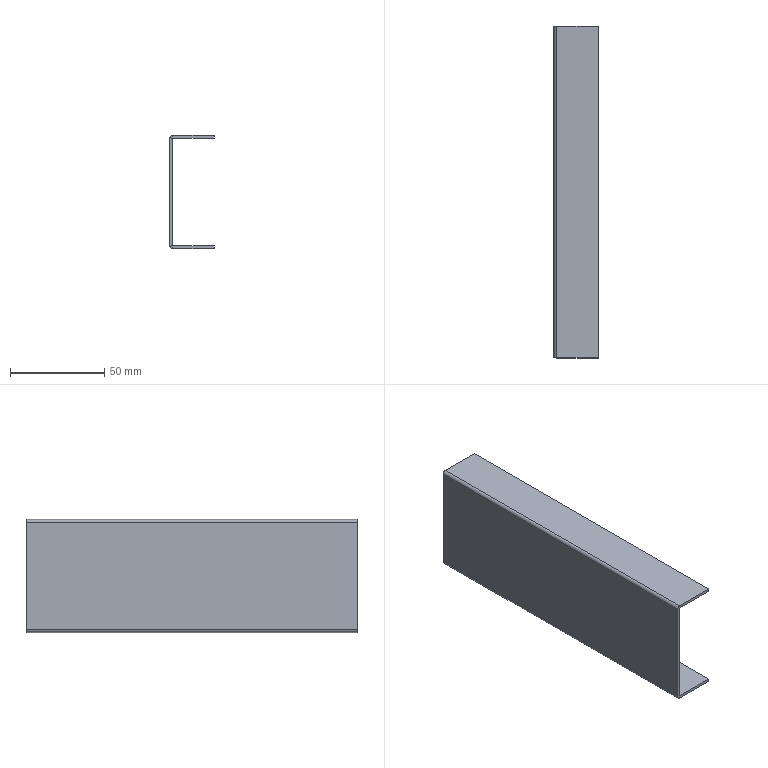Part | SolidWorks | features SplitBody 1 | 1 solid | 22 faces | box 23.5 x 176 x 60 mm | volume 27263 mm3 | plane 18 | cylinder 4 | commonest cylinder face diameters 0.2 x2 3.2 x2
STEP:
#1=CARTESIAN_POINT('',(3.,1360.,273.4));
#2=VERTEX_POINT('',#1);
#3=CARTESIAN_POINT('',(1.5,1360.,273.4));
#4=VERTEX_POINT('',#3);
#5=CARTESIAN_POINT('',(3.,1360.,273.4));
#6=DIRECTION('',(-1.,0.,0.));
#7=VECTOR('',#6,1000.);
#8=LINE('',#5,#7);
#9=EDGE_CURVE('',#2,#4,#8,.T.);
#10=ORIENTED_EDGE('',*,*,#9,.T.);
#11=CARTESIAN_POINT('',(1.5,1360.,216.6));
#12=VERTEX_POINT('',#11);
#13=CARTESIAN_POINT('',(1.5,1360.,0.));
#14=DIRECTION('',(0.,0.,1.));
#15=VECTOR('',#14,1000.);
#16=LINE('',#13,#15);
#17=EDGE_CURVE('',#12,#4,#16,.T.);
#18=ORIENTED_EDGE('',*,*,#17,.F.);
#19=CARTESIAN_POINT('',(3.,1360.,216.6));
#20=VERTEX_POINT('',#19);
#21=CARTESIAN_POINT('',(3.,1360.,216.6));
#22=DIRECTION('',(-1.,0.,0.));
#23=VECTOR('',#22,1000.);
#24=LINE('',#21,#23);
#25=EDGE_CURVE('',#20,#12,#24,.T.);
#26=ORIENTED_EDGE('',*,*,#25,.F.);
#27=CARTESIAN_POINT('',(3.,1360.,275.));
#28=DIRECTION('',(0.,0.,1.));
#29=VECTOR('',#28,1000.);
#30=LINE('',#27,#29);
#31=EDGE_CURVE('',#20,#2,#30,.T.);
#32=ORIENTED_EDGE('',*,*,#31,.T.);
#33=EDGE_LOOP('',(#10,#18,#26,#32));
#34=FACE_OUTER_BOUND('',#33,.T.);
#35=CARTESIAN_POINT('',(1.5,1360.,275.));
#36=DIRECTION('',(0.,1.,0.));
#37=DIRECTION('',(-1.,0.,0.));
#38=AXIS2_PLACEMENT_3D('',#35,#36,#37);
#39=PLANE('',#38);
#40=ADVANCED_FACE('',(#34),#39,.F.);
#41=CARTESIAN_POINT('',(3.,1536.,273.4));
#42=VERTEX_POINT('',#41);
#43=CARTESIAN_POINT('',(1.5,1536.,273.4));
#44=VERTEX_POINT('',#43);
#45=CARTESIAN_POINT('',(3.,1536.,273.4));
#46=DIRECTION('',(-1.,0.,0.));
#47=VECTOR('',#46,1000.);
#48=LINE('',#45,#47);
#49=EDGE_CURVE('',#42,#44,#48,.T.);
#50=ORIENTED_EDGE('',*,*,#49,.F.);
#51=CARTESIAN_POINT('',(3.,1536.,216.6));
#52=VERTEX_POINT('',#51);
#53=CARTESIAN_POINT('',(3.,1536.,216.5));
#54=DIRECTION('',(0.,0.,-1.));
#55=VECTOR('',#54,1000.);
#56=LINE('',#53,#55);
#57=EDGE_CURVE('',#42,#52,#56,.T.);
#58=ORIENTED_EDGE('',*,*,#57,.T.);
#59=CARTESIAN_POINT('',(1.5,1536.,216.6));
#60=VERTEX_POINT('',#59);
#61=CARTESIAN_POINT('',(1.5,1536.,216.6));
#62=DIRECTION('',(-1.,0.,0.));
#63=VECTOR('',#62,1000.);
#64=LINE('',#61,#63);
#65=EDGE_CURVE('',#52,#60,#64,.T.);
#66=ORIENTED_EDGE('',*,*,#65,.T.);
#67=CARTESIAN_POINT('',(1.5,1536.,0.));
#68=DIRECTION('',(0.,0.,-1.));
#69=VECTOR('',#68,1000.);
#70=LINE('',#67,#69);
#71=EDGE_CURVE('',#44,#60,#70,.T.);
#72=ORIENTED_EDGE('',*,*,#71,.F.);
#73=EDGE_LOOP('',(#50,#58,#66,#72));
#74=FACE_OUTER_BOUND('',#73,.T.);
#75=CARTESIAN_POINT('',(1.5,1536.,216.5));
#76=DIRECTION('',(0.,-1.,0.));
#77=DIRECTION('',(1.,0.,0.));
#78=AXIS2_PLACEMENT_3D('',#75,#76,#77);
#79=PLANE('',#78);
#80=ADVANCED_FACE('',(#74),#79,.F.);
#81=CARTESIAN_POINT('',(1.5,1360.,273.4));
#82=DIRECTION('',(0.,1.,0.));
#83=VECTOR('',#82,1000.);
#84=LINE('',#81,#83);
#85=EDGE_CURVE('',#4,#44,#84,.T.);
#86=ORIENTED_EDGE('',*,*,#85,.T.);
#87=ORIENTED_EDGE('',*,*,#71,.T.);
#88=CARTESIAN_POINT('',(1.5,1536.,216.6));
#89=DIRECTION('',(0.,1.,0.));
#90=VECTOR('',#89,1000.);
#91=LINE('',#88,#90);
#92=EDGE_CURVE('',#12,#60,#91,.T.);
#93=ORIENTED_EDGE('',*,*,#92,.F.);
#94=ORIENTED_EDGE('',*,*,#17,.T.);
#95=EDGE_LOOP('',(#86,#87,#93,#94));
#96=FACE_OUTER_BOUND('',#95,.T.);
#97=CARTESIAN_POINT('',(1.5,0.,0.));
#98=DIRECTION('',(1.,0.,0.));
#99=DIRECTION('',(0.,0.,-1.));
#100=AXIS2_PLACEMENT_3D('',#97,#98,#99);
#101=PLANE('',#100);
#102=ADVANCED_FACE('',(#96),#101,.F.);
#103=ORIENTED_EDGE('',*,*,#57,.F.);
#104=CARTESIAN_POINT('',(3.,1360.,273.4));
#105=DIRECTION('',(0.,1.,0.));
#106=VECTOR('',#105,1000.);
#107=LINE('',#104,#106);
#108=EDGE_CURVE('',#2,#42,#107,.T.);
#109=ORIENTED_EDGE('',*,*,#108,.F.);
#110=ORIENTED_EDGE('',*,*,#31,.F.);
#111=CARTESIAN_POINT('',(3.,1536.,216.6));
#112=DIRECTION('',(0.,-1.,0.));
#113=VECTOR('',#112,1000.);
#114=LINE('',#111,#113);
#115=EDGE_CURVE('',#52,#20,#114,.T.);
#116=ORIENTED_EDGE('',*,*,#115,.F.);
#117=EDGE_LOOP('',(#103,#109,#110,#116));
#118=FACE_OUTER_BOUND('',#117,.T.);
#119=CARTESIAN_POINT('',(3.,0.,0.));
#120=DIRECTION('',(1.,0.,0.));
#121=DIRECTION('',(0.,0.,-1.));
#122=AXIS2_PLACEMENT_3D('',#119,#120,#121);
#123=PLANE('',#122);
#124=ADVANCED_FACE('',(#118),#123,.T.);
#125=CARTESIAN_POINT('',(3.1,1536.,216.5));
#126=VERTEX_POINT('',#125);
#127=CARTESIAN_POINT('',(3.1,1536.,215.));
#128=VERTEX_POINT('',#127);
#129=CARTESIAN_POINT('',(3.1,1536.,216.5));
#130=DIRECTION('',(0.,0.,-1.));
#131=VECTOR('',#130,1000.);
#132=LINE('',#129,#131);
#133=EDGE_CURVE('',#126,#128,#132,.T.);
#134=ORIENTED_EDGE('',*,*,#133,.F.);
#135=CARTESIAN_POINT('',(25.,1536.,216.5));
#136=VERTEX_POINT('',#135);
#137=CARTESIAN_POINT('',(25.,1536.,216.5));
#138=DIRECTION('',(-1.,0.,0.));
#139=VECTOR('',#138,1000.);
#140=LINE('',#137,#139);
#141=EDGE_CURVE('',#136,#126,#140,.T.);
#142=ORIENTED_EDGE('',*,*,#141,.F.);
#143=CARTESIAN_POINT('',(25.,1536.,215.));
#144=VERTEX_POINT('',#143);
#145=CARTESIAN_POINT('',(25.,1536.,216.5));
#146=DIRECTION('',(0.,0.,-1.));
#147=VECTOR('',#146,1000.);
#148=LINE('',#145,#147);
#149=EDGE_CURVE('',#136,#144,#148,.T.);
#150=ORIENTED_EDGE('',*,*,#149,.T.);
#151=CARTESIAN_POINT('',(25.,1536.,215.));
#152=DIRECTION('',(-1.,0.,0.));
#153=VECTOR('',#152,1000.);
#154=LINE('',#151,#153);
#155=EDGE_CURVE('',#144,#128,#154,.T.);
#156=ORIENTED_EDGE('',*,*,#155,.T.);
#157=EDGE_LOOP('',(#134,#142,#150,#156));
#158=FACE_OUTER_BOUND('',#157,.T.);
#159=CARTESIAN_POINT('',(25.,1536.,216.5));
#160=DIRECTION('',(0.,-1.,0.));
#161=DIRECTION('',(0.,0.,-1.));
#162=AXIS2_PLACEMENT_3D('',#159,#160,#161);
#163=PLANE('',#162);
#164=ADVANCED_FACE('',(#158),#163,.F.);
#165=CARTESIAN_POINT('',(3.1,1360.,216.5));
#166=VERTEX_POINT('',#165);
#167=CARTESIAN_POINT('',(3.1,1360.,215.));
#168=VERTEX_POINT('',#167);
#169=CARTESIAN_POINT('',(3.1,1360.,216.5));
#170=DIRECTION('',(0.,0.,-1.));
#171=VECTOR('',#170,1000.);
#172=LINE('',#169,#171);
#173=EDGE_CURVE('',#166,#168,#172,.T.);
#174=ORIENTED_EDGE('',*,*,#173,.T.);
#175=CARTESIAN_POINT('',(25.,1360.,215.));
#176=VERTEX_POINT('',#175);
#177=CARTESIAN_POINT('',(25.,1360.,215.));
#178=DIRECTION('',(1.,0.,0.));
#179=VECTOR('',#178,1000.);
#180=LINE('',#177,#179);
#181=EDGE_CURVE('',#168,#176,#180,.T.);
#182=ORIENTED_EDGE('',*,*,#181,.T.);
#183=CARTESIAN_POINT('',(25.,1360.,216.5));
#184=VERTEX_POINT('',#183);
#185=CARTESIAN_POINT('',(25.,1360.,216.5));
#186=DIRECTION('',(0.,0.,-1.));
#187=VECTOR('',#186,1000.);
#188=LINE('',#185,#187);
#189=EDGE_CURVE('',#184,#176,#188,.T.);
#190=ORIENTED_EDGE('',*,*,#189,.F.);
#191=CARTESIAN_POINT('',(25.,1360.,216.5));
#192=DIRECTION('',(1.,0.,0.));
#193=VECTOR('',#192,1000.);
#194=LINE('',#191,#193);
#195=EDGE_CURVE('',#166,#184,#194,.T.);
#196=ORIENTED_EDGE('',*,*,#195,.F.);
#197=EDGE_LOOP('',(#174,#182,#190,#196));
#198=FACE_OUTER_BOUND('',#197,.T.);
#199=CARTESIAN_POINT('',(25.,1360.,216.5));
#200=DIRECTION('',(0.,1.,0.));
#201=DIRECTION('',(0.,0.,1.));
#202=AXIS2_PLACEMENT_3D('',#199,#200,#201);
#203=PLANE('',#202);
#204=ADVANCED_FACE('',(#198),#203,.F.);
#205=CARTESIAN_POINT('',(3.1,1360.,216.5));
#206=DIRECTION('',(0.,1.,0.));
#207=VECTOR('',#206,1000.);
#208=LINE('',#205,#207);
#209=EDGE_CURVE('',#166,#126,#208,.T.);
#210=ORIENTED_EDGE('',*,*,#209,.F.);
#211=ORIENTED_EDGE('',*,*,#195,.T.);
#212=CARTESIAN_POINT('',(25.,1536.,216.5));
#213=DIRECTION('',(0.,1.,0.));
#214=VECTOR('',#213,1000.);
#215=LINE('',#212,#214);
#216=EDGE_CURVE('',#184,#136,#215,.T.);
#217=ORIENTED_EDGE('',*,*,#216,.T.);
#218=ORIENTED_EDGE('',*,*,#141,.T.);
#219=EDGE_LOOP('',(#210,#211,#217,#218));
#220=FACE_OUTER_BOUND('',#219,.T.);
#221=CARTESIAN_POINT('',(0.,0.,216.5));
#222=DIRECTION('',(0.,0.,-1.));
#223=DIRECTION('',(-1.,0.,0.));
#224=AXIS2_PLACEMENT_3D('',#221,#222,#223);
#225=PLANE('',#224);
#226=ADVANCED_FACE('',(#220),#225,.F.);
#227=ORIENTED_EDGE('',*,*,#181,.F.);
#228=CARTESIAN_POINT('',(3.1,1360.,215.));
#229=DIRECTION('',(0.,1.,0.));
#230=VECTOR('',#229,1000.);
#231=LINE('',#228,#230);
#232=EDGE_CURVE('',#168,#128,#231,.T.);
#233=ORIENTED_EDGE('',*,*,#232,.T.);
#234=ORIENTED_EDGE('',*,*,#155,.F.);
#235=CARTESIAN_POINT('',(25.,1536.,215.));
#236=DIRECTION('',(0.,1.,0.));
#237=VECTOR('',#236,1000.);
#238=LINE('',#235,#237);
#239=EDGE_CURVE('',#176,#144,#238,.T.);
#240=ORIENTED_EDGE('',*,*,#239,.F.);
#241=EDGE_LOOP('',(#227,#233,#234,#240));
#242=FACE_OUTER_BOUND('',#241,.T.);
#243=CARTESIAN_POINT('',(0.,0.,215.));
#244=DIRECTION('',(0.,0.,-1.));
#245=DIRECTION('',(-1.,0.,0.));
#246=AXIS2_PLACEMENT_3D('',#243,#244,#245);
#247=PLANE('',#246);
#248=ADVANCED_FACE('',(#242),#247,.T.);
#249=ORIENTED_EDGE('',*,*,#239,.T.);
#250=ORIENTED_EDGE('',*,*,#149,.F.);
#251=ORIENTED_EDGE('',*,*,#216,.F.);
#252=ORIENTED_EDGE('',*,*,#189,.T.);
#253=EDGE_LOOP('',(#249,#250,#251,#252));
#254=FACE_OUTER_BOUND('',#253,.T.);
#255=CARTESIAN_POINT('',(25.,1536.,216.5));
#256=DIRECTION('',(-1.,0.,0.));
#257=DIRECTION('',(0.,-1.,0.));
#258=AXIS2_PLACEMENT_3D('',#255,#256,#257);
#259=PLANE('',#258);
#260=ADVANCED_FACE('',(#254),#259,.F.);
#261=ORIENTED_EDGE('',*,*,#65,.F.);
#262=CARTESIAN_POINT('',(3.1,1536.,216.6));
#263=DIRECTION('',(0.,1.,0.));
#264=DIRECTION('',(0.,0.,-1.));
#265=AXIS2_PLACEMENT_3D('',#262,#263,#264);
#266=CIRCLE('',#265,0.1);
#267=EDGE_CURVE('',#126,#52,#266,.T.);
#268=ORIENTED_EDGE('',*,*,#267,.F.);
#269=ORIENTED_EDGE('',*,*,#133,.T.);
#270=CARTESIAN_POINT('',(3.1,1536.,216.6));
#271=DIRECTION('',(0.,1.,0.));
#272=DIRECTION('',(0.,0.,-1.));
#273=AXIS2_PLACEMENT_3D('',#270,#271,#272);
#274=CIRCLE('',#273,1.6);
#275=EDGE_CURVE('',#128,#60,#274,.T.);
#276=ORIENTED_EDGE('',*,*,#275,.T.);
#277=EDGE_LOOP('',(#261,#268,#269,#276));
#278=FACE_OUTER_BOUND('',#277,.T.);
#279=CARTESIAN_POINT('',(3.1,1536.,216.6));
#280=DIRECTION('',(0.,1.,0.));
#281=DIRECTION('',(0.,0.,1.));
#282=AXIS2_PLACEMENT_3D('',#279,#280,#281);
#283=PLANE('',#282);
#284=ADVANCED_FACE('',(#278),#283,.T.);
#285=CARTESIAN_POINT('',(3.1,1360.,216.6));
#286=DIRECTION('',(0.,-1.,0.));
#287=DIRECTION('',(0.,0.,-1.));
#288=AXIS2_PLACEMENT_3D('',#285,#286,#287);
#289=CIRCLE('',#288,0.1);
#290=EDGE_CURVE('',#20,#166,#289,.T.);
#291=ORIENTED_EDGE('',*,*,#290,.F.);
#292=ORIENTED_EDGE('',*,*,#25,.T.);
#293=CARTESIAN_POINT('',(3.1,1360.,216.6));
#294=DIRECTION('',(0.,-1.,0.));
#295=DIRECTION('',(0.,0.,-1.));
#296=AXIS2_PLACEMENT_3D('',#293,#294,#295);
#297=CIRCLE('',#296,1.6);
#298=EDGE_CURVE('',#12,#168,#297,.T.);
#299=ORIENTED_EDGE('',*,*,#298,.T.);
#300=ORIENTED_EDGE('',*,*,#173,.F.);
#301=EDGE_LOOP('',(#291,#292,#299,#300));
#302=FACE_OUTER_BOUND('',#301,.T.);
#303=CARTESIAN_POINT('',(3.1,1360.,216.6));
#304=DIRECTION('',(0.,1.,0.));
#305=DIRECTION('',(0.,0.,1.));
#306=AXIS2_PLACEMENT_3D('',#303,#304,#305);
#307=PLANE('',#306);
#308=ADVANCED_FACE('',(#302),#307,.F.);
#309=ORIENTED_EDGE('',*,*,#232,.F.);
#310=ORIENTED_EDGE('',*,*,#298,.F.);
#311=ORIENTED_EDGE('',*,*,#92,.T.);
#312=ORIENTED_EDGE('',*,*,#275,.F.);
#313=EDGE_LOOP('',(#309,#310,#311,#312));
#314=FACE_OUTER_BOUND('',#313,.T.);
#315=CARTESIAN_POINT('',(3.1,1360.,216.6));
#316=DIRECTION('',(0.,-1.,0.));
#317=DIRECTION('',(-1.,0.,0.));
#318=AXIS2_PLACEMENT_3D('',#315,#316,#317);
#319=CYLINDRICAL_SURFACE('',#318,1.6);
#320=ADVANCED_FACE('',(#314),#319,.T.);
#321=ORIENTED_EDGE('',*,*,#209,.T.);
#322=ORIENTED_EDGE('',*,*,#267,.T.);
#323=ORIENTED_EDGE('',*,*,#115,.T.);
#324=ORIENTED_EDGE('',*,*,#290,.T.);
#325=EDGE_LOOP('',(#321,#322,#323,#324));
#326=FACE_OUTER_BOUND('',#325,.T.);
#327=CARTESIAN_POINT('',(3.1,1360.,216.6));
#328=DIRECTION('',(0.,-1.,0.));
#329=DIRECTION('',(-1.,0.,0.));
#330=AXIS2_PLACEMENT_3D('',#327,#328,#329);
#331=CYLINDRICAL_SURFACE('',#330,0.1);
#332=ADVANCED_FACE('',(#326),#331,.F.);
#333=CARTESIAN_POINT('',(3.1,1536.,273.5));
#334=VERTEX_POINT('',#333);
#335=CARTESIAN_POINT('',(3.1,1536.,275.));
#336=VERTEX_POINT('',#335);
#337=CARTESIAN_POINT('',(3.1,1536.,275.));
#338=DIRECTION('',(0.,0.,1.));
#339=VECTOR('',#338,1000.);
#340=LINE('',#337,#339);
#341=EDGE_CURVE('',#334,#336,#340,.T.);
#342=ORIENTED_EDGE('',*,*,#341,.F.);
#343=CARTESIAN_POINT('',(3.1,1536.,273.4));
#344=DIRECTION('',(0.,1.,0.));
#345=DIRECTION('',(0.,0.,-1.));
#346=AXIS2_PLACEMENT_3D('',#343,#344,#345);
#347=CIRCLE('',#346,0.1);
#348=EDGE_CURVE('',#42,#334,#347,.T.);
#349=ORIENTED_EDGE('',*,*,#348,.F.);
#350=ORIENTED_EDGE('',*,*,#49,.T.);
#351=CARTESIAN_POINT('',(3.1,1536.,273.4));
#352=DIRECTION('',(0.,1.,0.));
#353=DIRECTION('',(0.,0.,-1.));
#354=AXIS2_PLACEMENT_3D('',#351,#352,#353);
#355=CIRCLE('',#354,1.6);
#356=EDGE_CURVE('',#44,#336,#355,.T.);
#357=ORIENTED_EDGE('',*,*,#356,.T.);
#358=EDGE_LOOP('',(#342,#349,#350,#357));
#359=FACE_OUTER_BOUND('',#358,.T.);
#360=CARTESIAN_POINT('',(3.1,1536.,273.4));
#361=DIRECTION('',(0.,1.,0.));
#362=DIRECTION('',(0.,0.,1.));
#363=AXIS2_PLACEMENT_3D('',#360,#361,#362);
#364=PLANE('',#363);
#365=ADVANCED_FACE('',(#359),#364,.T.);
#366=CARTESIAN_POINT('',(3.1,1360.,273.5));
#367=VERTEX_POINT('',#366);
#368=CARTESIAN_POINT('',(3.1,1360.,273.4));
#369=DIRECTION('',(0.,-1.,0.));
#370=DIRECTION('',(0.,0.,-1.));
#371=AXIS2_PLACEMENT_3D('',#368,#369,#370);
#372=CIRCLE('',#371,0.1);
#373=EDGE_CURVE('',#367,#2,#372,.T.);
#374=ORIENTED_EDGE('',*,*,#373,.F.);
#375=CARTESIAN_POINT('',(3.1,1360.,275.));
#376=VERTEX_POINT('',#375);
#377=CARTESIAN_POINT('',(3.1,1360.,273.5));
#378=DIRECTION('',(0.,0.,1.));
#379=VECTOR('',#378,1000.);
#380=LINE('',#377,#379);
#381=EDGE_CURVE('',#367,#376,#380,.T.);
#382=ORIENTED_EDGE('',*,*,#381,.T.);
#383=CARTESIAN_POINT('',(3.1,1360.,273.4));
#384=DIRECTION('',(0.,-1.,0.));
#385=DIRECTION('',(0.,0.,-1.));
#386=AXIS2_PLACEMENT_3D('',#383,#384,#385);
#387=CIRCLE('',#386,1.6);
#388=EDGE_CURVE('',#376,#4,#387,.T.);
#389=ORIENTED_EDGE('',*,*,#388,.T.);
#390=ORIENTED_EDGE('',*,*,#9,.F.);
#391=EDGE_LOOP('',(#374,#382,#389,#390));
#392=FACE_OUTER_BOUND('',#391,.T.);
#393=CARTESIAN_POINT('',(3.1,1360.,273.4));
#394=DIRECTION('',(0.,1.,0.));
#395=DIRECTION('',(0.,0.,1.));
#396=AXIS2_PLACEMENT_3D('',#393,#394,#395);
#397=PLANE('',#396);
#398=ADVANCED_FACE('',(#392),#397,.F.);
#399=ORIENTED_EDGE('',*,*,#85,.F.);
#400=ORIENTED_EDGE('',*,*,#388,.F.);
#401=CARTESIAN_POINT('',(3.1,1536.,275.));
#402=DIRECTION('',(0.,1.,0.));
#403=VECTOR('',#402,1000.);
#404=LINE('',#401,#403);
#405=EDGE_CURVE('',#376,#336,#404,.T.);
#406=ORIENTED_EDGE('',*,*,#405,.T.);
#407=ORIENTED_EDGE('',*,*,#356,.F.);
#408=EDGE_LOOP('',(#399,#400,#406,#407));
#409=FACE_OUTER_BOUND('',#408,.T.);
#410=CARTESIAN_POINT('',(3.1,1360.,273.4));
#411=DIRECTION('',(0.,-1.,0.));
#412=DIRECTION('',(0.,0.,1.));
#413=AXIS2_PLACEMENT_3D('',#410,#411,#412);
#414=CYLINDRICAL_SURFACE('',#413,1.6);
#415=ADVANCED_FACE('',(#409),#414,.T.);
#416=ORIENTED_EDGE('',*,*,#108,.T.);
#417=ORIENTED_EDGE('',*,*,#348,.T.);
#418=CARTESIAN_POINT('',(3.1,1536.,273.5));
#419=DIRECTION('',(0.,-1.,0.));
#420=VECTOR('',#419,1000.);
#421=LINE('',#418,#420);
#422=EDGE_CURVE('',#334,#367,#421,.T.);
#423=ORIENTED_EDGE('',*,*,#422,.T.);
#424=ORIENTED_EDGE('',*,*,#373,.T.);
#425=EDGE_LOOP('',(#416,#417,#423,#424));
#426=FACE_OUTER_BOUND('',#425,.T.);
#427=CARTESIAN_POINT('',(3.1,1360.,273.4));
#428=DIRECTION('',(0.,-1.,0.));
#429=DIRECTION('',(0.,0.,1.));
#430=AXIS2_PLACEMENT_3D('',#427,#428,#429);
#431=CYLINDRICAL_SURFACE('',#430,0.1);
#432=ADVANCED_FACE('',(#426),#431,.F.);
#433=ORIENTED_EDGE('',*,*,#381,.F.);
#434=CARTESIAN_POINT('',(25.,1360.,273.5));
#435=VERTEX_POINT('',#434);
#436=CARTESIAN_POINT('',(25.,1360.,273.5));
#437=DIRECTION('',(1.,0.,0.));
#438=VECTOR('',#437,1000.);
#439=LINE('',#436,#438);
#440=EDGE_CURVE('',#367,#435,#439,.T.);
#441=ORIENTED_EDGE('',*,*,#440,.T.);
#442=CARTESIAN_POINT('',(25.,1360.,275.));
#443=VERTEX_POINT('',#442);
#444=CARTESIAN_POINT('',(25.,1360.,275.));
#445=DIRECTION('',(0.,0.,-1.));
#446=VECTOR('',#445,1000.);
#447=LINE('',#444,#446);
#448=EDGE_CURVE('',#443,#435,#447,.T.);
#449=ORIENTED_EDGE('',*,*,#448,.F.);
#450=CARTESIAN_POINT('',(0.,1360.,275.));
#451=DIRECTION('',(1.,0.,0.));
#452=VECTOR('',#451,1000.);
#453=LINE('',#450,#452);
#454=EDGE_CURVE('',#376,#443,#453,.T.);
#455=ORIENTED_EDGE('',*,*,#454,.F.);
#456=EDGE_LOOP('',(#433,#441,#449,#455));
#457=FACE_OUTER_BOUND('',#456,.T.);
#458=CARTESIAN_POINT('',(25.,1360.,275.));
#459=DIRECTION('',(0.,1.,0.));
#460=DIRECTION('',(0.,0.,1.));
#461=AXIS2_PLACEMENT_3D('',#458,#459,#460);
#462=PLANE('',#461);
#463=ADVANCED_FACE('',(#457),#462,.F.);
#464=ORIENTED_EDGE('',*,*,#341,.T.);
#465=CARTESIAN_POINT('',(25.,1536.,275.));
#466=VERTEX_POINT('',#465);
#467=CARTESIAN_POINT('',(0.,1536.,275.));
#468=DIRECTION('',(-1.,0.,0.));
#469=VECTOR('',#468,1000.);
#470=LINE('',#467,#469);
#471=EDGE_CURVE('',#466,#336,#470,.T.);
#472=ORIENTED_EDGE('',*,*,#471,.F.);
#473=CARTESIAN_POINT('',(25.,1536.,273.5));
#474=VERTEX_POINT('',#473);
#475=CARTESIAN_POINT('',(25.,1536.,275.));
#476=DIRECTION('',(0.,0.,-1.));
#477=VECTOR('',#476,1000.);
#478=LINE('',#475,#477);
#479=EDGE_CURVE('',#466,#474,#478,.T.);
#480=ORIENTED_EDGE('',*,*,#479,.T.);
#481=CARTESIAN_POINT('',(3.,1536.,273.5));
#482=DIRECTION('',(-1.,0.,0.));
#483=VECTOR('',#482,1000.);
#484=LINE('',#481,#483);
#485=EDGE_CURVE('',#474,#334,#484,.T.);
#486=ORIENTED_EDGE('',*,*,#485,.T.);
#487=EDGE_LOOP('',(#464,#472,#480,#486));
#488=FACE_OUTER_BOUND('',#487,.T.);
#489=CARTESIAN_POINT('',(3.,1536.,275.));
#490=DIRECTION('',(0.,-1.,0.));
#491=DIRECTION('',(0.,0.,-1.));
#492=AXIS2_PLACEMENT_3D('',#489,#490,#491);
#493=PLANE('',#492);
#494=ADVANCED_FACE('',(#488),#493,.F.);
#495=ORIENTED_EDGE('',*,*,#405,.F.);
#496=ORIENTED_EDGE('',*,*,#454,.T.);
#497=CARTESIAN_POINT('',(25.,0.,275.));
#498=DIRECTION('',(0.,1.,0.));
#499=VECTOR('',#498,1000.);
#500=LINE('',#497,#499);
#501=EDGE_CURVE('',#443,#466,#500,.T.);
#502=ORIENTED_EDGE('',*,*,#501,.T.);
#503=ORIENTED_EDGE('',*,*,#471,.T.);
#504=EDGE_LOOP('',(#495,#496,#502,#503));
#505=FACE_OUTER_BOUND('',#504,.T.);
#506=CARTESIAN_POINT('',(0.,0.,275.));
#507=DIRECTION('',(0.,0.,-1.));
#508=DIRECTION('',(-1.,0.,0.));
#509=AXIS2_PLACEMENT_3D('',#506,#507,#508);
#510=PLANE('',#509);
#511=ADVANCED_FACE('',(#505),#510,.F.);
#512=ORIENTED_EDGE('',*,*,#440,.F.);
#513=ORIENTED_EDGE('',*,*,#422,.F.);
#514=ORIENTED_EDGE('',*,*,#485,.F.);
#515=CARTESIAN_POINT('',(25.,1536.,273.5));
#516=DIRECTION('',(0.,1.,0.));
#517=VECTOR('',#516,1000.);
#518=LINE('',#515,#517);
#519=EDGE_CURVE('',#435,#474,#518,.T.);
#520=ORIENTED_EDGE('',*,*,#519,.F.);
#521=EDGE_LOOP('',(#512,#513,#514,#520));
#522=FACE_OUTER_BOUND('',#521,.T.);
#523=CARTESIAN_POINT('',(0.,0.,273.5));
#524=DIRECTION('',(0.,0.,-1.));
#525=DIRECTION('',(-1.,0.,0.));
#526=AXIS2_PLACEMENT_3D('',#523,#524,#525);
#527=PLANE('',#526);
#528=ADVANCED_FACE('',(#522),#527,.T.);
#529=ORIENTED_EDGE('',*,*,#519,.T.);
#530=ORIENTED_EDGE('',*,*,#479,.F.);
#531=ORIENTED_EDGE('',*,*,#501,.F.);
#532=ORIENTED_EDGE('',*,*,#448,.T.);
#533=EDGE_LOOP('',(#529,#530,#531,#532));
#534=FACE_OUTER_BOUND('',#533,.T.);
#535=CARTESIAN_POINT('',(25.,1536.,275.));
#536=DIRECTION('',(-1.,0.,0.));
#537=DIRECTION('',(0.,0.,1.));
#538=AXIS2_PLACEMENT_3D('',#535,#536,#537);
#539=PLANE('',#538);
#540=ADVANCED_FACE('',(#534),#539,.F.);
#541=CLOSED_SHELL('',(#40,#80,#102,#124,#164,#204,#226,#248,#260,#284,#308,#320,#332,#365,#398,#415,#432,#463,#494,#511,#528,#540));
#542=MANIFOLD_SOLID_BREP('',#541);
#543=CARTESIAN_POINT('',(0.,0.,0.));
#544=DIRECTION('',(0.,0.,1.));
#545=DIRECTION('',(1.,0.,0.));
#546=AXIS2_PLACEMENT_3D('',#543,#544,#545);
#547=(LENGTH_UNIT()NAMED_UNIT(*)SI_UNIT(.MILLI.,.METRE.));
#548=UNCERTAINTY_MEASURE_WITH_UNIT(LENGTH_MEASURE(0.00001),#547,'','');
#549=(NAMED_UNIT(*)PLANE_ANGLE_UNIT()SI_UNIT($,.RADIAN.));
#550=(NAMED_UNIT(*)SI_UNIT($,.STERADIAN.)SOLID_ANGLE_UNIT());
#551=(GEOMETRIC_REPRESENTATION_CONTEXT(3)GLOBAL_UNCERTAINTY_ASSIGNED_CONTEXT((#548))GLOBAL_UNIT_ASSIGNED_CONTEXT((#547,#549,#550))REPRESENTATION_CONTEXT('',''));
#552=ADVANCED_BREP_SHAPE_REPRESENTATION('',(#542,#546),#551);